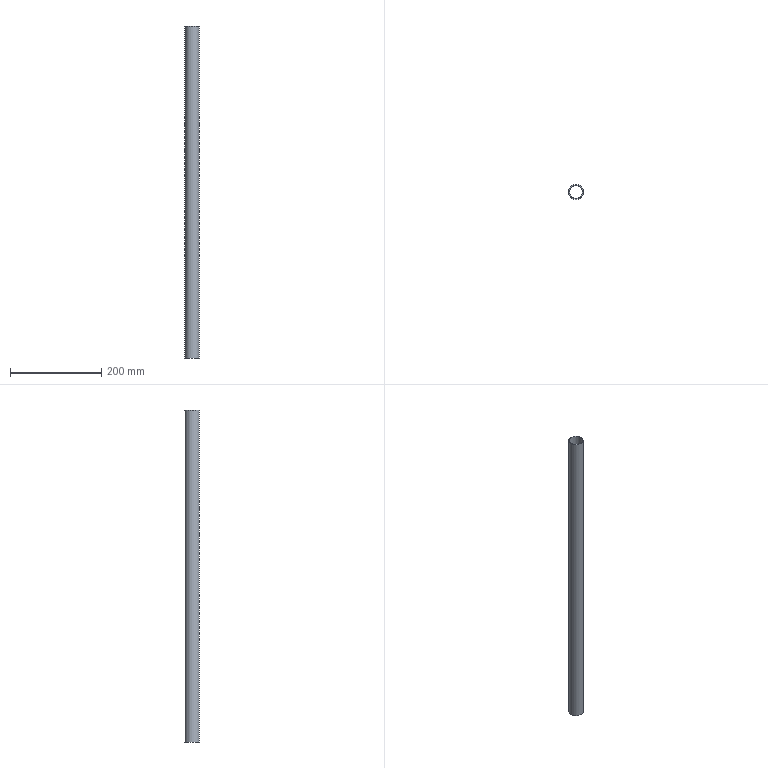Part | STEP file | Q7C1301 | 1 solid | 4 faces | box 31.8 x 31.8 x 726 mm | volume 103662 mm3 | plane 2 | cylinder 2 | commonest cylinder face diameters 28.8 x1 31.8 x1
STEP:
#1=CARTESIAN_POINT('',(0.,0.,0.));
#2=DIRECTION('',(0.,0.,1.));
#3=DIRECTION('',(1.,0.,0.));
#4=AXIS2_PLACEMENT_3D('',#1,#2,#3);
#5=CARTESIAN_POINT('',(15.9,0.,363.));
#6=VERTEX_POINT('',#5);
#7=CARTESIAN_POINT('',(0.,0.,363.));
#8=DIRECTION('',(0.,0.,1.));
#9=DIRECTION('',(1.,0.,0.));
#10=AXIS2_PLACEMENT_3D('',#7,#8,#9);
#11=CIRCLE('',#10,15.9);
#12=CARTESIAN_POINT('',(0.,0.,363.));
#13=DIRECTION('',(0.,0.,1.));
#14=DIRECTION('',(1.,0.,0.));
#15=AXIS2_PLACEMENT_3D('',#12,#13,#14);
#16=PLANE('',#15);
#17=CARTESIAN_POINT('',(0.,0.));
#18=DIRECTION('',(1.,0.));
#19=AXIS2_PLACEMENT_2D('',#17,#18);
#20=CIRCLE('',#19,15.9);
#21=(GEOMETRIC_REPRESENTATION_CONTEXT(2)PARAMETRIC_REPRESENTATION_CONTEXT()REPRESENTATION_CONTEXT('',''));
#22=DEFINITIONAL_REPRESENTATION('',(#20),#21);
#23=PCURVE('',#16,#22);
#24=CARTESIAN_POINT('',(0.,0.,363.));
#25=DIRECTION('',(0.,0.,-1.));
#26=DIRECTION('',(-1.,0.,0.));
#27=AXIS2_PLACEMENT_3D('',#24,#25,#26);
#28=CYLINDRICAL_SURFACE('',#27,15.9);
#29=CARTESIAN_POINT('',(9.425,0.));
#30=DIRECTION('',(-1.,0.));
#31=VECTOR('',#30,1.);
#32=LINE('',#29,#31);
#33=(GEOMETRIC_REPRESENTATION_CONTEXT(2)PARAMETRIC_REPRESENTATION_CONTEXT()REPRESENTATION_CONTEXT('',''));
#34=DEFINITIONAL_REPRESENTATION('',(#32),#33);
#35=PCURVE('',#28,#34);
#36=SURFACE_CURVE('',#11,(#23,#35),.PCURVE_S1.);
#37=EDGE_CURVE('',#6,#6,#36,.T.);
#38=ORIENTED_EDGE('',*,*,#37,.T.);
#39=EDGE_LOOP('',(#38));
#40=FACE_BOUND('',#39,.T.);
#41=CARTESIAN_POINT('',(14.4,0.,363.));
#42=VERTEX_POINT('',#41);
#43=CARTESIAN_POINT('',(0.,0.,363.));
#44=DIRECTION('',(0.,0.,1.));
#45=DIRECTION('',(1.,0.,0.));
#46=AXIS2_PLACEMENT_3D('',#43,#44,#45);
#47=CIRCLE('',#46,14.4);
#48=CARTESIAN_POINT('',(0.,0.));
#49=DIRECTION('',(1.,0.));
#50=AXIS2_PLACEMENT_2D('',#48,#49);
#51=CIRCLE('',#50,14.4);
#52=(GEOMETRIC_REPRESENTATION_CONTEXT(2)PARAMETRIC_REPRESENTATION_CONTEXT()REPRESENTATION_CONTEXT('',''));
#53=DEFINITIONAL_REPRESENTATION('',(#51),#52);
#54=PCURVE('',#16,#53);
#55=CARTESIAN_POINT('',(0.,0.,363.));
#56=DIRECTION('',(0.,0.,-1.));
#57=DIRECTION('',(-1.,0.,0.));
#58=AXIS2_PLACEMENT_3D('',#55,#56,#57);
#59=CYLINDRICAL_SURFACE('',#58,14.4);
#60=CARTESIAN_POINT('',(9.425,0.));
#61=DIRECTION('',(-1.,0.));
#62=VECTOR('',#61,1.);
#63=LINE('',#60,#62);
#64=(GEOMETRIC_REPRESENTATION_CONTEXT(2)PARAMETRIC_REPRESENTATION_CONTEXT()REPRESENTATION_CONTEXT('',''));
#65=DEFINITIONAL_REPRESENTATION('',(#63),#64);
#66=PCURVE('',#59,#65);
#67=SURFACE_CURVE('',#47,(#54,#66),.PCURVE_S1.);
#68=EDGE_CURVE('',#42,#42,#67,.T.);
#69=ORIENTED_EDGE('',*,*,#68,.F.);
#70=EDGE_LOOP('',(#69));
#71=FACE_BOUND('',#70,.T.);
#72=ADVANCED_FACE('',(#40,#71),#16,.T.);
#73=CARTESIAN_POINT('',(15.9,0.,-363.));
#74=VERTEX_POINT('',#73);
#75=CARTESIAN_POINT('',(0.,0.,-363.));
#76=DIRECTION('',(0.,0.,1.));
#77=DIRECTION('',(1.,0.,0.));
#78=AXIS2_PLACEMENT_3D('',#75,#76,#77);
#79=CIRCLE('',#78,15.9);
#80=CARTESIAN_POINT('',(0.,0.,-363.));
#81=DIRECTION('',(0.,0.,1.));
#82=DIRECTION('',(1.,0.,0.));
#83=AXIS2_PLACEMENT_3D('',#80,#81,#82);
#84=PLANE('',#83);
#85=CARTESIAN_POINT('',(0.,0.));
#86=DIRECTION('',(1.,0.));
#87=AXIS2_PLACEMENT_2D('',#85,#86);
#88=CIRCLE('',#87,15.9);
#89=(GEOMETRIC_REPRESENTATION_CONTEXT(2)PARAMETRIC_REPRESENTATION_CONTEXT()REPRESENTATION_CONTEXT('',''));
#90=DEFINITIONAL_REPRESENTATION('',(#88),#89);
#91=PCURVE('',#84,#90);
#92=CARTESIAN_POINT('',(9.425,726.));
#93=DIRECTION('',(-1.,0.));
#94=VECTOR('',#93,1.);
#95=LINE('',#92,#94);
#96=(GEOMETRIC_REPRESENTATION_CONTEXT(2)PARAMETRIC_REPRESENTATION_CONTEXT()REPRESENTATION_CONTEXT('',''));
#97=DEFINITIONAL_REPRESENTATION('',(#95),#96);
#98=PCURVE('',#28,#97);
#99=SURFACE_CURVE('',#79,(#91,#98),.PCURVE_S1.);
#100=EDGE_CURVE('',#74,#74,#99,.T.);
#101=ORIENTED_EDGE('',*,*,#100,.F.);
#102=EDGE_LOOP('',(#101));
#103=FACE_BOUND('',#102,.T.);
#104=CARTESIAN_POINT('',(14.4,0.,-363.));
#105=VERTEX_POINT('',#104);
#106=CARTESIAN_POINT('',(0.,0.,-363.));
#107=DIRECTION('',(0.,0.,1.));
#108=DIRECTION('',(1.,0.,0.));
#109=AXIS2_PLACEMENT_3D('',#106,#107,#108);
#110=CIRCLE('',#109,14.4);
#111=CARTESIAN_POINT('',(0.,0.));
#112=DIRECTION('',(1.,0.));
#113=AXIS2_PLACEMENT_2D('',#111,#112);
#114=CIRCLE('',#113,14.4);
#115=(GEOMETRIC_REPRESENTATION_CONTEXT(2)PARAMETRIC_REPRESENTATION_CONTEXT()REPRESENTATION_CONTEXT('',''));
#116=DEFINITIONAL_REPRESENTATION('',(#114),#115);
#117=PCURVE('',#84,#116);
#118=CARTESIAN_POINT('',(9.425,726.));
#119=DIRECTION('',(-1.,0.));
#120=VECTOR('',#119,1.);
#121=LINE('',#118,#120);
#122=(GEOMETRIC_REPRESENTATION_CONTEXT(2)PARAMETRIC_REPRESENTATION_CONTEXT()REPRESENTATION_CONTEXT('',''));
#123=DEFINITIONAL_REPRESENTATION('',(#121),#122);
#124=PCURVE('',#59,#123);
#125=SURFACE_CURVE('',#110,(#117,#124),.PCURVE_S1.);
#126=EDGE_CURVE('',#105,#105,#125,.T.);
#127=ORIENTED_EDGE('',*,*,#126,.T.);
#128=EDGE_LOOP('',(#127));
#129=FACE_BOUND('',#128,.T.);
#130=ADVANCED_FACE('',(#103,#129),#84,.F.);
#131=ORIENTED_EDGE('',*,*,#37,.F.);
#132=CARTESIAN_POINT('',(15.9,0.,363.));
#133=CARTESIAN_POINT('',(15.9,0.,-363.));
#134=B_SPLINE_CURVE_WITH_KNOTS('',1,(#132,#133),.UNSPECIFIED.,.F.,.F.,(2,2),(0.,726.),.PIECEWISE_BEZIER_KNOTS.);
#135=CARTESIAN_POINT('',(9.425,0.));
#136=DIRECTION('',(0.,1.));
#137=VECTOR('',#136,1.);
#138=LINE('',#135,#137);
#139=(GEOMETRIC_REPRESENTATION_CONTEXT(2)PARAMETRIC_REPRESENTATION_CONTEXT()REPRESENTATION_CONTEXT('',''));
#140=DEFINITIONAL_REPRESENTATION('',(#138),#139);
#141=PCURVE('',#28,#140);
#142=CARTESIAN_POINT('',(3.142,0.));
#143=DIRECTION('',(0.,1.));
#144=VECTOR('',#143,1.);
#145=LINE('',#142,#144);
#146=(GEOMETRIC_REPRESENTATION_CONTEXT(2)PARAMETRIC_REPRESENTATION_CONTEXT()REPRESENTATION_CONTEXT('',''));
#147=DEFINITIONAL_REPRESENTATION('',(#145),#146);
#148=PCURVE('',#28,#147);
#149=SEAM_CURVE('',#134,(#141,#148),.PCURVE_S1.);
#150=EDGE_CURVE('',#6,#74,#149,.T.);
#151=ORIENTED_EDGE('',*,*,#150,.T.);
#152=ORIENTED_EDGE('',*,*,#100,.T.);
#153=ORIENTED_EDGE('',*,*,#150,.F.);
#154=EDGE_LOOP('',(#131,#151,#152,#153));
#155=FACE_BOUND('',#154,.T.);
#156=ADVANCED_FACE('',(#155),#28,.T.);
#157=ORIENTED_EDGE('',*,*,#68,.F.);
#158=CARTESIAN_POINT('',(14.4,0.,363.));
#159=CARTESIAN_POINT('',(14.4,0.,-363.));
#160=B_SPLINE_CURVE_WITH_KNOTS('',1,(#158,#159),.UNSPECIFIED.,.F.,.F.,(2,2),(0.,726.),.PIECEWISE_BEZIER_KNOTS.);
#161=CARTESIAN_POINT('',(9.425,0.));
#162=DIRECTION('',(0.,1.));
#163=VECTOR('',#162,1.);
#164=LINE('',#161,#163);
#165=(GEOMETRIC_REPRESENTATION_CONTEXT(2)PARAMETRIC_REPRESENTATION_CONTEXT()REPRESENTATION_CONTEXT('',''));
#166=DEFINITIONAL_REPRESENTATION('',(#164),#165);
#167=PCURVE('',#59,#166);
#168=CARTESIAN_POINT('',(3.142,0.));
#169=DIRECTION('',(0.,1.));
#170=VECTOR('',#169,1.);
#171=LINE('',#168,#170);
#172=(GEOMETRIC_REPRESENTATION_CONTEXT(2)PARAMETRIC_REPRESENTATION_CONTEXT()REPRESENTATION_CONTEXT('',''));
#173=DEFINITIONAL_REPRESENTATION('',(#171),#172);
#174=PCURVE('',#59,#173);
#175=SEAM_CURVE('',#160,(#167,#174),.PCURVE_S1.);
#176=EDGE_CURVE('',#42,#105,#175,.T.);
#177=ORIENTED_EDGE('',*,*,#176,.T.);
#178=ORIENTED_EDGE('',*,*,#126,.T.);
#179=ORIENTED_EDGE('',*,*,#176,.F.);
#180=EDGE_LOOP('',(#157,#177,#178,#179));
#181=FACE_BOUND('',#180,.F.);
#182=ADVANCED_FACE('',(#181),#59,.F.);
#183=CLOSED_SHELL('',(#72,#130,#156,#182));
#184=MANIFOLD_SOLID_BREP('',#183);
#185=(LENGTH_UNIT()NAMED_UNIT(*)SI_UNIT(.MILLI.,.METRE.));
#186=UNCERTAINTY_MEASURE_WITH_UNIT(LENGTH_MEASURE(0.00001),#185,'','');
#187=(NAMED_UNIT(*)PLANE_ANGLE_UNIT()SI_UNIT($,.RADIAN.));
#188=(NAMED_UNIT(*)SI_UNIT($,.STERADIAN.)SOLID_ANGLE_UNIT());
#189=(GEOMETRIC_REPRESENTATION_CONTEXT(3)GLOBAL_UNCERTAINTY_ASSIGNED_CONTEXT((#186))GLOBAL_UNIT_ASSIGNED_CONTEXT((#185,#187,#188))REPRESENTATION_CONTEXT('',''));
#190=ADVANCED_BREP_SHAPE_REPRESENTATION('',(#4,#184),#189);